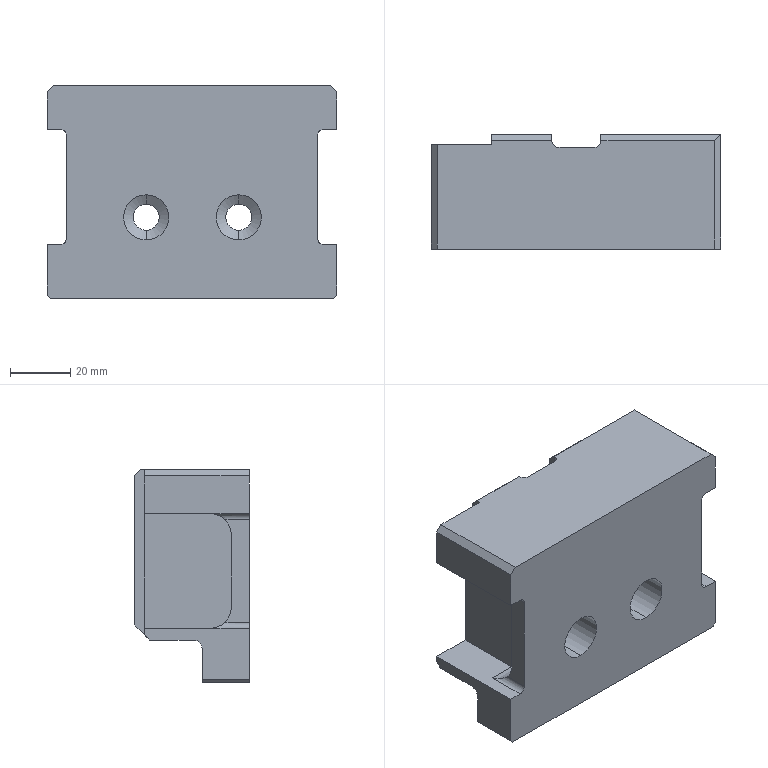Part | STEP file | 1_id118_x_t | 1 solid | 56 faces | box 96 x 38 x 70.5 mm | volume 174436 mm3 | plane 33 | cylinder 19 | cone 4 | commonest cylinder face diameters 4 x6 8.65 x4 14 x4 15 x4 6 x1